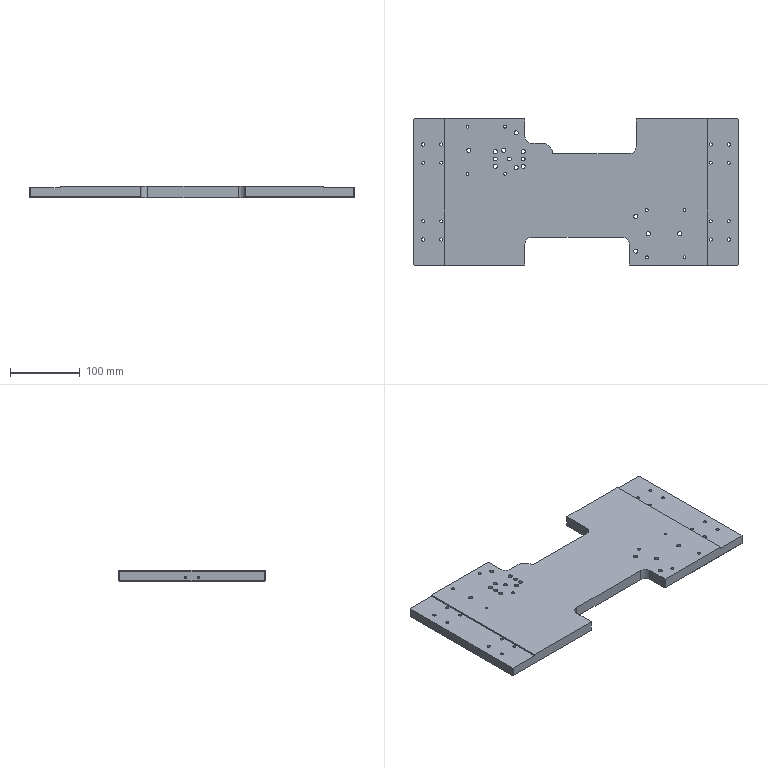Part | 1 solid | 218 faces | box 467 x 210 x 16 mm | volume 1301573 mm3 | cylinder 144 | plane 50 | cone 24 | commonest cylinder face diameters 4.5 x32 8 x32 3.3 x24 6 x24 4.2 x16 5.5 x6